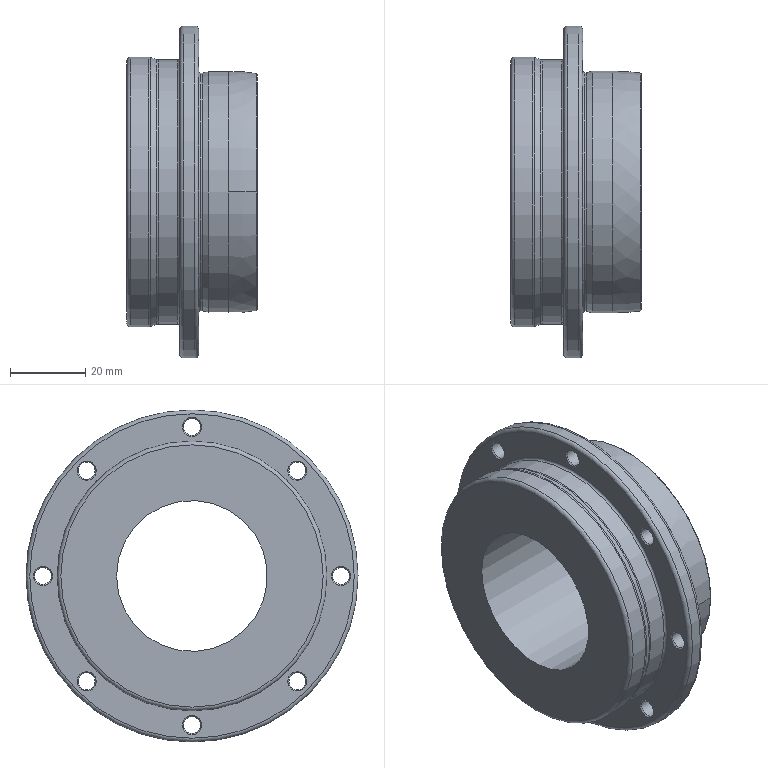Part | STEP file | P0278200003_D | 1 solid | 47 faces | box 34.5 x 88 x 88 mm | volume 90794 mm3 | cone 18 | cylinder 14 | torus 9 | plane 4 | spline 2 | commonest cylinder face diameters 4.5 x8 40 x1 63.2 x1 64 x1 70 x1 71.5 x1